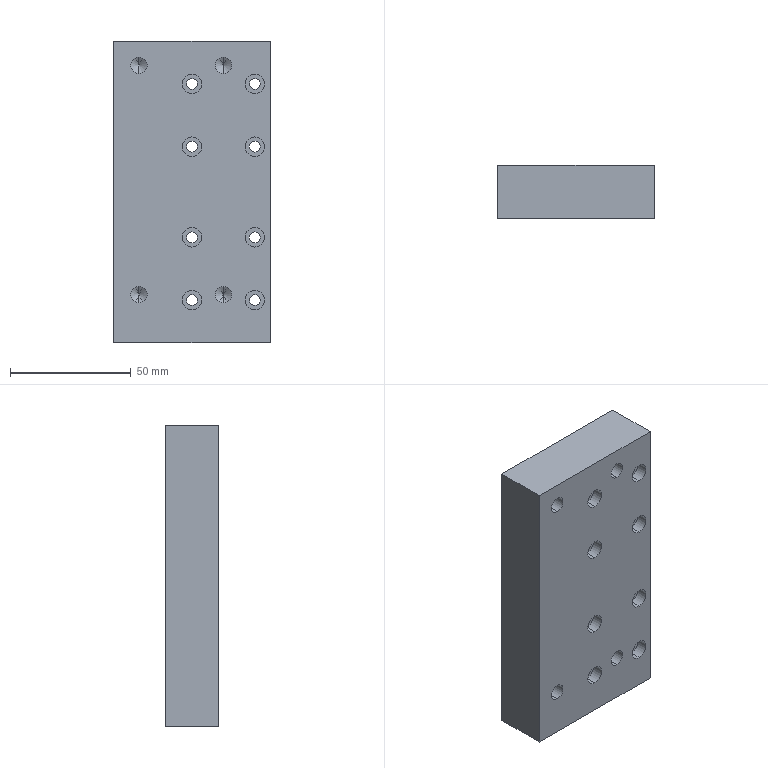Part | STEP file | X77-07005Z | 1 solid | 62 faces | box 65 x 22 x 125 mm | volume 171718 mm3 | cylinder 40 | plane 14 | cone 8 | commonest cylinder face diameters 4.5 x16 8 x16 6.8 x8